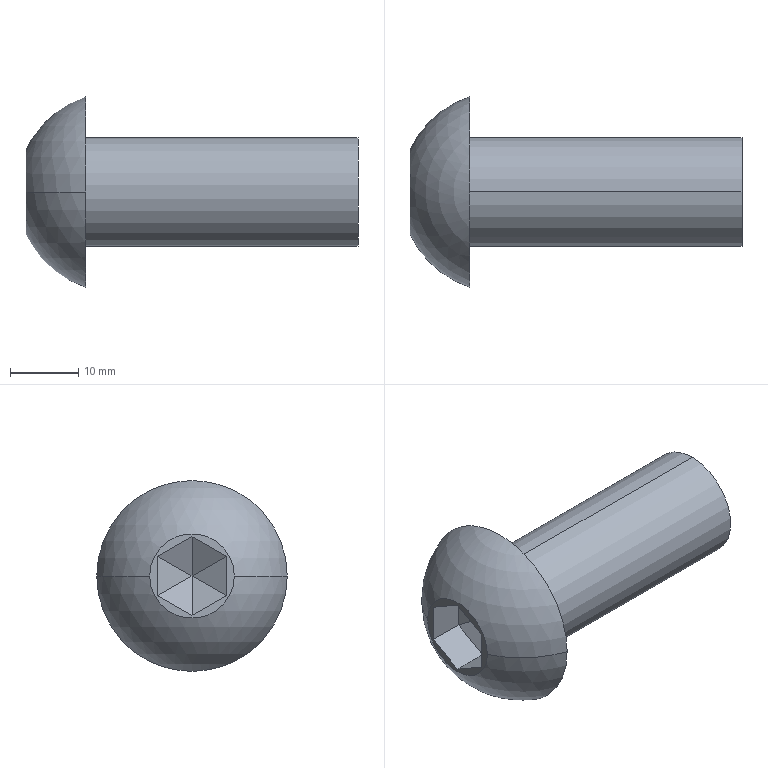Part | SolidWorks | features Cut 2, RevCut 2, Boss 1, Extrusion 1, Fillet 1, LPattern 1 | 1 solid | 19 faces | box 48.8 x 28 x 28 mm | volume 11109 mm3 | plane 15 | sphere 2 | cylinder 2 | commonest cylinder face diameters 16 x2
STEP:
#1=CARTESIAN_POINT('',(8.8,14.,0.));
#2=VERTEX_POINT('',#1);
#3=CARTESIAN_POINT('',(8.8,-14.,0.));
#4=VERTEX_POINT('',#3);
#5=CARTESIAN_POINT('',(8.8,0.,0.));
#6=DIRECTION('',(-1.,0.,0.));
#7=DIRECTION('',(0.,0.,1.));
#8=AXIS2_PLACEMENT_3D('',#5,#6,#7);
#9=CIRCLE('',#8,14.);
#10=EDGE_CURVE('',#2,#4,#9,.T.);
#11=ORIENTED_EDGE('',*,*,#10,.T.);
#12=CARTESIAN_POINT('',(0.,-6.215,0.));
#13=VERTEX_POINT('',#12);
#14=CARTESIAN_POINT('',(13.342,0.,0.));
#15=DIRECTION('',(0.,0.,-1.));
#16=DIRECTION('',(0.,1.,0.));
#17=AXIS2_PLACEMENT_3D('',#14,#15,#16);
#18=CIRCLE('',#17,14.718);
#19=EDGE_CURVE('',#4,#13,#18,.T.);
#20=ORIENTED_EDGE('',*,*,#19,.T.);
#21=CARTESIAN_POINT('',(0.,6.215,0.));
#22=VERTEX_POINT('',#21);
#23=CARTESIAN_POINT('',(0.,0.,0.));
#24=DIRECTION('',(-1.,0.,0.));
#25=DIRECTION('',(0.,0.,1.));
#26=AXIS2_PLACEMENT_3D('',#23,#24,#25);
#27=CIRCLE('',#26,6.215);
#28=EDGE_CURVE('',#22,#13,#27,.T.);
#29=ORIENTED_EDGE('',*,*,#28,.F.);
#30=CARTESIAN_POINT('',(13.342,0.,0.));
#31=DIRECTION('',(0.,0.,1.));
#32=DIRECTION('',(1.,0.,0.));
#33=AXIS2_PLACEMENT_3D('',#30,#31,#32);
#34=CIRCLE('',#33,14.718);
#35=EDGE_CURVE('',#2,#22,#34,.T.);
#36=ORIENTED_EDGE('',*,*,#35,.F.);
#37=EDGE_LOOP('',(#11,#20,#29,#36));
#38=FACE_OUTER_BOUND('',#37,.T.);
#39=CARTESIAN_POINT('',(13.342,0.,0.));
#40=DIRECTION('',(0.,0.,-1.));
#41=DIRECTION('',(0.,1.,0.));
#42=AXIS2_PLACEMENT_3D('',#39,#40,#41);
#43=SPHERICAL_SURFACE('',#42,14.718);
#44=ADVANCED_FACE('',(#38),#43,.T.);
#45=CARTESIAN_POINT('',(48.8,0.,-8.));
#46=VERTEX_POINT('',#45);
#47=CARTESIAN_POINT('',(48.8,0.,8.));
#48=VERTEX_POINT('',#47);
#49=CARTESIAN_POINT('',(48.8,0.,0.));
#50=DIRECTION('',(1.,0.,0.));
#51=DIRECTION('',(0.,0.,-1.));
#52=AXIS2_PLACEMENT_3D('',#49,#50,#51);
#53=CIRCLE('',#52,8.);
#54=EDGE_CURVE('',#46,#48,#53,.T.);
#55=ORIENTED_EDGE('',*,*,#54,.F.);
#56=CARTESIAN_POINT('',(8.8,0.,-8.));
#57=VERTEX_POINT('',#56);
#58=CARTESIAN_POINT('',(48.8,0.,-8.));
#59=DIRECTION('',(-1.,0.,0.));
#60=VECTOR('',#59,1000.);
#61=LINE('',#58,#60);
#62=EDGE_CURVE('',#46,#57,#61,.T.);
#63=ORIENTED_EDGE('',*,*,#62,.T.);
#64=CARTESIAN_POINT('',(8.8,0.,8.));
#65=VERTEX_POINT('',#64);
#66=CARTESIAN_POINT('',(8.8,0.,0.));
#67=DIRECTION('',(1.,0.,0.));
#68=DIRECTION('',(0.,0.,-1.));
#69=AXIS2_PLACEMENT_3D('',#66,#67,#68);
#70=CIRCLE('',#69,8.);
#71=EDGE_CURVE('',#57,#65,#70,.T.);
#72=ORIENTED_EDGE('',*,*,#71,.T.);
#73=CARTESIAN_POINT('',(48.8,0.,8.));
#74=DIRECTION('',(-1.,0.,0.));
#75=VECTOR('',#74,1000.);
#76=LINE('',#73,#75);
#77=EDGE_CURVE('',#48,#65,#76,.T.);
#78=ORIENTED_EDGE('',*,*,#77,.F.);
#79=EDGE_LOOP('',(#55,#63,#72,#78));
#80=FACE_OUTER_BOUND('',#79,.T.);
#81=CARTESIAN_POINT('',(48.8,0.,0.));
#82=DIRECTION('',(-1.,0.,0.));
#83=DIRECTION('',(0.,0.,1.));
#84=AXIS2_PLACEMENT_3D('',#81,#82,#83);
#85=CYLINDRICAL_SURFACE('',#84,8.);
#86=ADVANCED_FACE('',(#80),#85,.T.);
#87=ORIENTED_EDGE('',*,*,#28,.T.);
#88=CARTESIAN_POINT('',(0.,0.,0.));
#89=DIRECTION('',(-1.,0.,0.));
#90=DIRECTION('',(0.,0.,1.));
#91=AXIS2_PLACEMENT_3D('',#88,#89,#90);
#92=CIRCLE('',#91,6.215);
#93=EDGE_CURVE('',#13,#22,#92,.T.);
#94=ORIENTED_EDGE('',*,*,#93,.T.);
#95=EDGE_LOOP('',(#87,#94));
#96=FACE_OUTER_BOUND('',#95,.T.);
#97=CARTESIAN_POINT('',(0.,-5.,-2.887));
#98=VERTEX_POINT('',#97);
#99=CARTESIAN_POINT('',(0.,0.,-5.774));
#100=VERTEX_POINT('',#99);
#101=CARTESIAN_POINT('',(0.,-5.,-2.887));
#102=DIRECTION('',(0.,0.866,-0.5));
#103=VECTOR('',#102,1000.);
#104=LINE('',#101,#103);
#105=EDGE_CURVE('',#98,#100,#104,.T.);
#106=ORIENTED_EDGE('',*,*,#105,.T.);
#107=CARTESIAN_POINT('',(0.,5.,-2.887));
#108=VERTEX_POINT('',#107);
#109=CARTESIAN_POINT('',(0.,0.,-5.774));
#110=DIRECTION('',(0.,0.866,0.5));
#111=VECTOR('',#110,1000.);
#112=LINE('',#109,#111);
#113=EDGE_CURVE('',#100,#108,#112,.T.);
#114=ORIENTED_EDGE('',*,*,#113,.T.);
#115=CARTESIAN_POINT('',(0.,5.,2.887));
#116=VERTEX_POINT('',#115);
#117=CARTESIAN_POINT('',(0.,5.,-2.887));
#118=DIRECTION('',(0.,0.,1.));
#119=VECTOR('',#118,1000.);
#120=LINE('',#117,#119);
#121=EDGE_CURVE('',#108,#116,#120,.T.);
#122=ORIENTED_EDGE('',*,*,#121,.T.);
#123=CARTESIAN_POINT('',(0.,0.,5.774));
#124=VERTEX_POINT('',#123);
#125=CARTESIAN_POINT('',(0.,5.,2.887));
#126=DIRECTION('',(0.,-0.866,0.5));
#127=VECTOR('',#126,1000.);
#128=LINE('',#125,#127);
#129=EDGE_CURVE('',#116,#124,#128,.T.);
#130=ORIENTED_EDGE('',*,*,#129,.T.);
#131=CARTESIAN_POINT('',(0.,-5.,2.887));
#132=VERTEX_POINT('',#131);
#133=CARTESIAN_POINT('',(0.,0.,5.774));
#134=DIRECTION('',(0.,-0.866,-0.5));
#135=VECTOR('',#134,1000.);
#136=LINE('',#133,#135);
#137=EDGE_CURVE('',#124,#132,#136,.T.);
#138=ORIENTED_EDGE('',*,*,#137,.T.);
#139=CARTESIAN_POINT('',(0.,-5.,2.887));
#140=DIRECTION('',(0.,0.,-1.));
#141=VECTOR('',#140,1000.);
#142=LINE('',#139,#141);
#143=EDGE_CURVE('',#132,#98,#142,.T.);
#144=ORIENTED_EDGE('',*,*,#143,.T.);
#145=EDGE_LOOP('',(#106,#114,#122,#130,#138,#144));
#146=FACE_BOUND('',#145,.T.);
#147=CARTESIAN_POINT('',(0.,0.,0.));
#148=DIRECTION('',(1.,0.,0.));
#149=DIRECTION('',(0.,0.,-1.));
#150=AXIS2_PLACEMENT_3D('',#147,#148,#149);
#151=PLANE('',#150);
#152=ADVANCED_FACE('',(#96,#146),#151,.F.);
#153=ORIENTED_EDGE('',*,*,#10,.F.);
#154=CARTESIAN_POINT('',(8.8,0.,0.));
#155=DIRECTION('',(-1.,0.,0.));
#156=DIRECTION('',(0.,0.,1.));
#157=AXIS2_PLACEMENT_3D('',#154,#155,#156);
#158=CIRCLE('',#157,14.);
#159=EDGE_CURVE('',#4,#2,#158,.T.);
#160=ORIENTED_EDGE('',*,*,#159,.F.);
#161=EDGE_LOOP('',(#153,#160));
#162=FACE_OUTER_BOUND('',#161,.T.);
#163=CARTESIAN_POINT('',(8.8,0.,0.));
#164=DIRECTION('',(1.,0.,0.));
#165=DIRECTION('',(0.,0.,-1.));
#166=AXIS2_PLACEMENT_3D('',#163,#164,#165);
#167=CIRCLE('',#166,8.);
#168=EDGE_CURVE('',#65,#57,#167,.T.);
#169=ORIENTED_EDGE('',*,*,#168,.F.);
#170=ORIENTED_EDGE('',*,*,#71,.F.);
#171=EDGE_LOOP('',(#169,#170));
#172=FACE_BOUND('',#171,.T.);
#173=CARTESIAN_POINT('',(8.8,0.,0.));
#174=DIRECTION('',(1.,0.,0.));
#175=DIRECTION('',(0.,0.,-1.));
#176=AXIS2_PLACEMENT_3D('',#173,#174,#175);
#177=PLANE('',#176);
#178=ADVANCED_FACE('',(#162,#172),#177,.T.);
#179=ORIENTED_EDGE('',*,*,#62,.F.);
#180=CARTESIAN_POINT('',(48.8,0.,0.));
#181=DIRECTION('',(1.,0.,0.));
#182=DIRECTION('',(0.,0.,-1.));
#183=AXIS2_PLACEMENT_3D('',#180,#181,#182);
#184=CIRCLE('',#183,8.);
#185=EDGE_CURVE('',#48,#46,#184,.T.);
#186=ORIENTED_EDGE('',*,*,#185,.F.);
#187=ORIENTED_EDGE('',*,*,#77,.T.);
#188=ORIENTED_EDGE('',*,*,#168,.T.);
#189=EDGE_LOOP('',(#179,#186,#187,#188));
#190=FACE_OUTER_BOUND('',#189,.T.);
#191=CARTESIAN_POINT('',(48.8,0.,0.));
#192=DIRECTION('',(-1.,0.,0.));
#193=DIRECTION('',(0.,0.,1.));
#194=AXIS2_PLACEMENT_3D('',#191,#192,#193);
#195=CYLINDRICAL_SURFACE('',#194,8.);
#196=ADVANCED_FACE('',(#190),#195,.T.);
#197=ORIENTED_EDGE('',*,*,#185,.T.);
#198=ORIENTED_EDGE('',*,*,#54,.T.);
#199=EDGE_LOOP('',(#197,#198));
#200=FACE_OUTER_BOUND('',#199,.T.);
#201=CARTESIAN_POINT('',(48.8,0.,0.));
#202=DIRECTION('',(1.,0.,0.));
#203=DIRECTION('',(0.,0.,-1.));
#204=AXIS2_PLACEMENT_3D('',#201,#202,#203);
#205=PLANE('',#204);
#206=ADVANCED_FACE('',(#200),#205,.T.);
#207=ORIENTED_EDGE('',*,*,#19,.F.);
#208=ORIENTED_EDGE('',*,*,#159,.T.);
#209=ORIENTED_EDGE('',*,*,#35,.T.);
#210=ORIENTED_EDGE('',*,*,#93,.F.);
#211=EDGE_LOOP('',(#207,#208,#209,#210));
#212=FACE_OUTER_BOUND('',#211,.T.);
#213=CARTESIAN_POINT('',(13.342,0.,0.));
#214=DIRECTION('',(0.,0.,-1.));
#215=DIRECTION('',(0.,1.,0.));
#216=AXIS2_PLACEMENT_3D('',#213,#214,#215);
#217=SPHERICAL_SURFACE('',#216,14.718);
#218=ADVANCED_FACE('',(#212),#217,.T.);
#219=ORIENTED_EDGE('',*,*,#105,.F.);
#220=CARTESIAN_POINT('',(5.2,-5.,-2.887));
#221=VERTEX_POINT('',#220);
#222=CARTESIAN_POINT('',(5.2,-5.,-2.887));
#223=DIRECTION('',(-1.,0.,0.));
#224=VECTOR('',#223,1000.);
#225=LINE('',#222,#224);
#226=EDGE_CURVE('',#221,#98,#225,.T.);
#227=ORIENTED_EDGE('',*,*,#226,.F.);
#228=CARTESIAN_POINT('',(5.2,0.,-5.774));
#229=VERTEX_POINT('',#228);
#230=CARTESIAN_POINT('',(5.2,-5.,-2.887));
#231=DIRECTION('',(0.,0.866,-0.5));
#232=VECTOR('',#231,1000.);
#233=LINE('',#230,#232);
#234=EDGE_CURVE('',#221,#229,#233,.T.);
#235=ORIENTED_EDGE('',*,*,#234,.T.);
#236=CARTESIAN_POINT('',(5.2,0.,-5.774));
#237=DIRECTION('',(-1.,0.,0.));
#238=VECTOR('',#237,1000.);
#239=LINE('',#236,#238);
#240=EDGE_CURVE('',#229,#100,#239,.T.);
#241=ORIENTED_EDGE('',*,*,#240,.T.);
#242=EDGE_LOOP('',(#219,#227,#235,#241));
#243=FACE_OUTER_BOUND('',#242,.T.);
#244=CARTESIAN_POINT('',(5.2,-5.,-2.887));
#245=DIRECTION('',(0.,0.5,0.866));
#246=DIRECTION('',(0.,-0.866,0.5));
#247=AXIS2_PLACEMENT_3D('',#244,#245,#246);
#248=PLANE('',#247);
#249=ADVANCED_FACE('',(#243),#248,.T.);
#250=ORIENTED_EDGE('',*,*,#113,.F.);
#251=ORIENTED_EDGE('',*,*,#240,.F.);
#252=CARTESIAN_POINT('',(5.2,5.,-2.887));
#253=VERTEX_POINT('',#252);
#254=CARTESIAN_POINT('',(5.2,0.,-5.774));
#255=DIRECTION('',(0.,0.866,0.5));
#256=VECTOR('',#255,1000.);
#257=LINE('',#254,#256);
#258=EDGE_CURVE('',#229,#253,#257,.T.);
#259=ORIENTED_EDGE('',*,*,#258,.T.);
#260=CARTESIAN_POINT('',(5.2,5.,-2.887));
#261=DIRECTION('',(-1.,0.,0.));
#262=VECTOR('',#261,1000.);
#263=LINE('',#260,#262);
#264=EDGE_CURVE('',#253,#108,#263,.T.);
#265=ORIENTED_EDGE('',*,*,#264,.T.);
#266=EDGE_LOOP('',(#250,#251,#259,#265));
#267=FACE_OUTER_BOUND('',#266,.T.);
#268=CARTESIAN_POINT('',(5.2,0.,-5.774));
#269=DIRECTION('',(0.,-0.5,0.866));
#270=DIRECTION('',(0.,-0.866,-0.5));
#271=AXIS2_PLACEMENT_3D('',#268,#269,#270);
#272=PLANE('',#271);
#273=ADVANCED_FACE('',(#267),#272,.T.);
#274=ORIENTED_EDGE('',*,*,#121,.F.);
#275=ORIENTED_EDGE('',*,*,#264,.F.);
#276=CARTESIAN_POINT('',(5.2,5.,2.887));
#277=VERTEX_POINT('',#276);
#278=CARTESIAN_POINT('',(5.2,5.,-2.887));
#279=DIRECTION('',(0.,0.,1.));
#280=VECTOR('',#279,1000.);
#281=LINE('',#278,#280);
#282=EDGE_CURVE('',#253,#277,#281,.T.);
#283=ORIENTED_EDGE('',*,*,#282,.T.);
#284=CARTESIAN_POINT('',(5.2,5.,2.887));
#285=DIRECTION('',(-1.,0.,0.));
#286=VECTOR('',#285,1000.);
#287=LINE('',#284,#286);
#288=EDGE_CURVE('',#277,#116,#287,.T.);
#289=ORIENTED_EDGE('',*,*,#288,.T.);
#290=EDGE_LOOP('',(#274,#275,#283,#289));
#291=FACE_OUTER_BOUND('',#290,.T.);
#292=CARTESIAN_POINT('',(5.2,5.,-2.887));
#293=DIRECTION('',(0.,-1.,0.));
#294=DIRECTION('',(0.,0.,-1.));
#295=AXIS2_PLACEMENT_3D('',#292,#293,#294);
#296=PLANE('',#295);
#297=ADVANCED_FACE('',(#291),#296,.T.);
#298=ORIENTED_EDGE('',*,*,#129,.F.);
#299=ORIENTED_EDGE('',*,*,#288,.F.);
#300=CARTESIAN_POINT('',(5.2,0.,5.774));
#301=VERTEX_POINT('',#300);
#302=CARTESIAN_POINT('',(5.2,5.,2.887));
#303=DIRECTION('',(0.,-0.866,0.5));
#304=VECTOR('',#303,1000.);
#305=LINE('',#302,#304);
#306=EDGE_CURVE('',#277,#301,#305,.T.);
#307=ORIENTED_EDGE('',*,*,#306,.T.);
#308=CARTESIAN_POINT('',(5.2,0.,5.774));
#309=DIRECTION('',(-1.,0.,0.));
#310=VECTOR('',#309,1000.);
#311=LINE('',#308,#310);
#312=EDGE_CURVE('',#301,#124,#311,.T.);
#313=ORIENTED_EDGE('',*,*,#312,.T.);
#314=EDGE_LOOP('',(#298,#299,#307,#313));
#315=FACE_OUTER_BOUND('',#314,.T.);
#316=CARTESIAN_POINT('',(5.2,5.,2.887));
#317=DIRECTION('',(0.,-0.5,-0.866));
#318=DIRECTION('',(0.,0.866,-0.5));
#319=AXIS2_PLACEMENT_3D('',#316,#317,#318);
#320=PLANE('',#319);
#321=ADVANCED_FACE('',(#315),#320,.T.);
#322=ORIENTED_EDGE('',*,*,#137,.F.);
#323=ORIENTED_EDGE('',*,*,#312,.F.);
#324=CARTESIAN_POINT('',(5.2,-5.,2.887));
#325=VERTEX_POINT('',#324);
#326=CARTESIAN_POINT('',(5.2,0.,5.774));
#327=DIRECTION('',(0.,-0.866,-0.5));
#328=VECTOR('',#327,1000.);
#329=LINE('',#326,#328);
#330=EDGE_CURVE('',#301,#325,#329,.T.);
#331=ORIENTED_EDGE('',*,*,#330,.T.);
#332=CARTESIAN_POINT('',(5.2,-5.,2.887));
#333=DIRECTION('',(-1.,0.,0.));
#334=VECTOR('',#333,1000.);
#335=LINE('',#332,#334);
#336=EDGE_CURVE('',#325,#132,#335,.T.);
#337=ORIENTED_EDGE('',*,*,#336,.T.);
#338=EDGE_LOOP('',(#322,#323,#331,#337));
#339=FACE_OUTER_BOUND('',#338,.T.);
#340=CARTESIAN_POINT('',(5.2,0.,5.774));
#341=DIRECTION('',(0.,0.5,-0.866));
#342=DIRECTION('',(0.,0.866,0.5));
#343=AXIS2_PLACEMENT_3D('',#340,#341,#342);
#344=PLANE('',#343);
#345=ADVANCED_FACE('',(#339),#344,.T.);
#346=ORIENTED_EDGE('',*,*,#143,.F.);
#347=ORIENTED_EDGE('',*,*,#336,.F.);
#348=CARTESIAN_POINT('',(5.2,-5.,2.887));
#349=DIRECTION('',(0.,0.,-1.));
#350=VECTOR('',#349,1000.);
#351=LINE('',#348,#350);
#352=EDGE_CURVE('',#325,#221,#351,.T.);
#353=ORIENTED_EDGE('',*,*,#352,.T.);
#354=ORIENTED_EDGE('',*,*,#226,.T.);
#355=EDGE_LOOP('',(#346,#347,#353,#354));
#356=FACE_OUTER_BOUND('',#355,.T.);
#357=CARTESIAN_POINT('',(5.2,-5.,2.887));
#358=DIRECTION('',(0.,1.,0.));
#359=DIRECTION('',(0.,0.,1.));
#360=AXIS2_PLACEMENT_3D('',#357,#358,#359);
#361=PLANE('',#360);
#362=ADVANCED_FACE('',(#356),#361,.T.);
#363=ORIENTED_EDGE('',*,*,#330,.F.);
#364=CARTESIAN_POINT('',(8.087,0.,0.));
#365=VERTEX_POINT('',#364);
#366=CARTESIAN_POINT('',(5.2,0.,5.774));
#367=DIRECTION('',(-0.4472,0.,0.8944));
#368=VECTOR('',#367,1000.);
#369=LINE('',#366,#368);
#370=EDGE_CURVE('',#365,#301,#369,.T.);
#371=ORIENTED_EDGE('',*,*,#370,.F.);
#372=CARTESIAN_POINT('',(5.2,-5.,2.887));
#373=DIRECTION('',(-0.4472,-0.7746,0.4472));
#374=VECTOR('',#373,1000.);
#375=LINE('',#372,#374);
#376=EDGE_CURVE('',#365,#325,#375,.T.);
#377=ORIENTED_EDGE('',*,*,#376,.T.);
#378=EDGE_LOOP('',(#363,#371,#377));
#379=FACE_OUTER_BOUND('',#378,.T.);
#380=CARTESIAN_POINT('',(5.2,0.,5.774));
#381=DIRECTION('',(0.866,-0.25,0.433));
#382=DIRECTION('',(0.4472,0.,-0.8944));
#383=AXIS2_PLACEMENT_3D('',#380,#381,#382);
#384=PLANE('',#383);
#385=ADVANCED_FACE('',(#379),#384,.F.);
#386=ORIENTED_EDGE('',*,*,#352,.F.);
#387=ORIENTED_EDGE('',*,*,#376,.F.);
#388=CARTESIAN_POINT('',(5.2,-5.,-2.887));
#389=DIRECTION('',(-0.4472,-0.7746,-0.4472));
#390=VECTOR('',#389,1000.);
#391=LINE('',#388,#390);
#392=EDGE_CURVE('',#365,#221,#391,.T.);
#393=ORIENTED_EDGE('',*,*,#392,.T.);
#394=EDGE_LOOP('',(#386,#387,#393));
#395=FACE_OUTER_BOUND('',#394,.T.);
#396=CARTESIAN_POINT('',(5.2,-5.,2.887));
#397=DIRECTION('',(0.866,-0.5,0.));
#398=DIRECTION('',(0.5,0.866,0.));
#399=AXIS2_PLACEMENT_3D('',#396,#397,#398);
#400=PLANE('',#399);
#401=ADVANCED_FACE('',(#395),#400,.F.);
#402=ORIENTED_EDGE('',*,*,#234,.F.);
#403=ORIENTED_EDGE('',*,*,#392,.F.);
#404=CARTESIAN_POINT('',(5.2,0.,-5.774));
#405=DIRECTION('',(-0.4472,0.,-0.8944));
#406=VECTOR('',#405,1000.);
#407=LINE('',#404,#406);
#408=EDGE_CURVE('',#365,#229,#407,.T.);
#409=ORIENTED_EDGE('',*,*,#408,.T.);
#410=EDGE_LOOP('',(#402,#403,#409));
#411=FACE_OUTER_BOUND('',#410,.T.);
#412=CARTESIAN_POINT('',(5.2,-5.,-2.887));
#413=DIRECTION('',(0.866,-0.25,-0.433));
#414=DIRECTION('',(-0.4472,0.,-0.8944));
#415=AXIS2_PLACEMENT_3D('',#412,#413,#414);
#416=PLANE('',#415);
#417=ADVANCED_FACE('',(#411),#416,.F.);
#418=ORIENTED_EDGE('',*,*,#258,.F.);
#419=ORIENTED_EDGE('',*,*,#408,.F.);
#420=CARTESIAN_POINT('',(5.2,5.,-2.887));
#421=DIRECTION('',(-0.4472,0.7746,-0.4472));
#422=VECTOR('',#421,1000.);
#423=LINE('',#420,#422);
#424=EDGE_CURVE('',#365,#253,#423,.T.);
#425=ORIENTED_EDGE('',*,*,#424,.T.);
#426=EDGE_LOOP('',(#418,#419,#425));
#427=FACE_OUTER_BOUND('',#426,.T.);
#428=CARTESIAN_POINT('',(5.2,0.,-5.774));
#429=DIRECTION('',(0.866,0.25,-0.433));
#430=DIRECTION('',(-0.4472,0.,-0.8944));
#431=AXIS2_PLACEMENT_3D('',#428,#429,#430);
#432=PLANE('',#431);
#433=ADVANCED_FACE('',(#427),#432,.F.);
#434=ORIENTED_EDGE('',*,*,#282,.F.);
#435=ORIENTED_EDGE('',*,*,#424,.F.);
#436=CARTESIAN_POINT('',(5.2,5.,2.887));
#437=DIRECTION('',(-0.4472,0.7746,0.4472));
#438=VECTOR('',#437,1000.);
#439=LINE('',#436,#438);
#440=EDGE_CURVE('',#365,#277,#439,.T.);
#441=ORIENTED_EDGE('',*,*,#440,.T.);
#442=EDGE_LOOP('',(#434,#435,#441));
#443=FACE_OUTER_BOUND('',#442,.T.);
#444=CARTESIAN_POINT('',(5.2,5.,-2.887));
#445=DIRECTION('',(0.866,0.5,0.));
#446=DIRECTION('',(-0.5,0.866,0.));
#447=AXIS2_PLACEMENT_3D('',#444,#445,#446);
#448=PLANE('',#447);
#449=ADVANCED_FACE('',(#443),#448,.F.);
#450=ORIENTED_EDGE('',*,*,#306,.F.);
#451=ORIENTED_EDGE('',*,*,#440,.F.);
#452=ORIENTED_EDGE('',*,*,#370,.T.);
#453=EDGE_LOOP('',(#450,#451,#452));
#454=FACE_OUTER_BOUND('',#453,.T.);
#455=CARTESIAN_POINT('',(5.2,5.,2.887));
#456=DIRECTION('',(0.866,0.25,0.433));
#457=DIRECTION('',(0.4472,0.,-0.8944));
#458=AXIS2_PLACEMENT_3D('',#455,#456,#457);
#459=PLANE('',#458);
#460=ADVANCED_FACE('',(#454),#459,.F.);
#461=CLOSED_SHELL('',(#44,#86,#152,#178,#196,#206,#218,#249,#273,#297,#321,#345,#362,#385,#401,#417,#433,#449,#460));
#462=MANIFOLD_SOLID_BREP('',#461);
#463=CARTESIAN_POINT('',(0.,0.,0.));
#464=DIRECTION('',(0.,0.,1.));
#465=DIRECTION('',(1.,0.,0.));
#466=AXIS2_PLACEMENT_3D('',#463,#464,#465);
#467=(LENGTH_UNIT()NAMED_UNIT(*)SI_UNIT(.MILLI.,.METRE.));
#468=UNCERTAINTY_MEASURE_WITH_UNIT(LENGTH_MEASURE(0.00001),#467,'','');
#469=(NAMED_UNIT(*)PLANE_ANGLE_UNIT()SI_UNIT($,.RADIAN.));
#470=(NAMED_UNIT(*)SI_UNIT($,.STERADIAN.)SOLID_ANGLE_UNIT());
#471=(GEOMETRIC_REPRESENTATION_CONTEXT(3)GLOBAL_UNCERTAINTY_ASSIGNED_CONTEXT((#468))GLOBAL_UNIT_ASSIGNED_CONTEXT((#467,#469,#470))REPRESENTATION_CONTEXT('',''));
#472=ADVANCED_BREP_SHAPE_REPRESENTATION('',(#462,#466),#471);